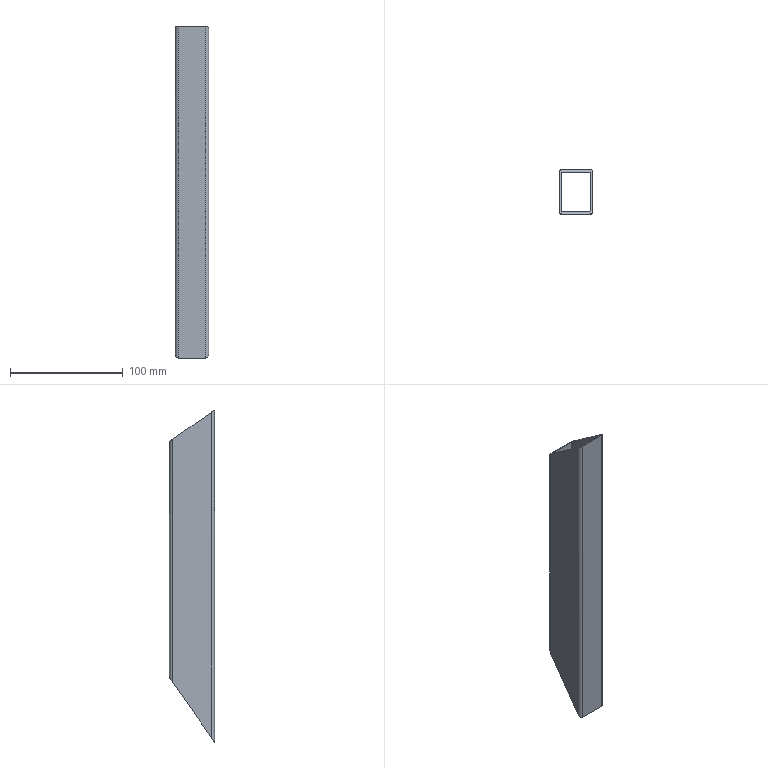Part | SolidWorks | features BaseBody 1 | 1 solid | 18 faces | box 30 x 40 x 295 mm | volume 80145 mm3 | plane 10 | cylinder 8 | commonest cylinder face diameters 1 x4 6 x4
STEP:
#1=CARTESIAN_POINT('',(-15.,17.,121.592));
#2=VERTEX_POINT('',#1);
#3=CARTESIAN_POINT('',(-15.,17.,-94.659));
#4=VERTEX_POINT('',#3);
#5=CARTESIAN_POINT('',(-15.,17.,147.5));
#6=DIRECTION('',(0.,0.,-1.));
#7=VECTOR('',#6,1000.);
#8=LINE('',#5,#7);
#9=EDGE_CURVE('',#2,#4,#8,.T.);
#10=ORIENTED_EDGE('',*,*,#9,.T.);
#11=CARTESIAN_POINT('',(-15.,-17.,-143.216));
#12=VERTEX_POINT('',#11);
#13=CARTESIAN_POINT('',(-15.,-20.,-147.5));
#14=DIRECTION('',(0.,0.5736,0.8192));
#15=VECTOR('',#14,1000.);
#16=LINE('',#13,#15);
#17=EDGE_CURVE('',#12,#4,#16,.T.);
#18=ORIENTED_EDGE('',*,*,#17,.F.);
#19=CARTESIAN_POINT('',(-15.,-17.,145.399));
#20=VERTEX_POINT('',#19);
#21=CARTESIAN_POINT('',(-15.,-17.,147.5));
#22=DIRECTION('',(0.,0.,-1.));
#23=VECTOR('',#22,1000.);
#24=LINE('',#21,#23);
#25=EDGE_CURVE('',#20,#12,#24,.T.);
#26=ORIENTED_EDGE('',*,*,#25,.F.);
#27=CARTESIAN_POINT('',(-15.,-20.,147.5));
#28=DIRECTION('',(0.,-0.8192,0.5736));
#29=VECTOR('',#28,1000.);
#30=LINE('',#27,#29);
#31=EDGE_CURVE('',#2,#20,#30,.T.);
#32=ORIENTED_EDGE('',*,*,#31,.F.);
#33=EDGE_LOOP('',(#10,#18,#26,#32));
#34=FACE_OUTER_BOUND('',#33,.T.);
#35=CARTESIAN_POINT('',(-15.,17.,147.5));
#36=DIRECTION('',(1.,0.,0.));
#37=DIRECTION('',(0.,1.,0.));
#38=AXIS2_PLACEMENT_3D('',#35,#36,#37);
#39=PLANE('',#38);
#40=ADVANCED_FACE('',(#34),#39,.F.);
#41=CARTESIAN_POINT('',(-12.,20.,119.492));
#42=VERTEX_POINT('',#41);
#43=CARTESIAN_POINT('',(-12.,20.,-90.374));
#44=VERTEX_POINT('',#43);
#45=CARTESIAN_POINT('',(-12.,20.,147.5));
#46=DIRECTION('',(0.,0.,-1.));
#47=VECTOR('',#46,1000.);
#48=LINE('',#45,#47);
#49=EDGE_CURVE('',#42,#44,#48,.T.);
#50=ORIENTED_EDGE('',*,*,#49,.T.);
#51=CARTESIAN_POINT('',(-12.,20.,-90.374));
#52=CARTESIAN_POINT('',(-13.757,20.,-90.374));
#53=CARTESIAN_POINT('',(-15.,18.757,-92.149));
#54=CARTESIAN_POINT('',(-15.,17.,-94.659));
#55=(BOUNDED_CURVE()B_SPLINE_CURVE(3,(#51,#52,#53,#54),.UNSPECIFIED.,.F.,.T.)B_SPLINE_CURVE_WITH_KNOTS((4,4),(3.142,4.712),.UNSPECIFIED.)CURVE()GEOMETRIC_REPRESENTATION_ITEM()RATIONAL_B_SPLINE_CURVE((1.,0.8047,0.8047,1.))REPRESENTATION_ITEM(''));
#56=EDGE_CURVE('',#44,#4,#55,.T.);
#57=ORIENTED_EDGE('',*,*,#56,.T.);
#58=ORIENTED_EDGE('',*,*,#9,.F.);
#59=CARTESIAN_POINT('',(-15.,17.,121.592));
#60=CARTESIAN_POINT('',(-15.,18.757,120.362));
#61=CARTESIAN_POINT('',(-13.757,20.,119.492));
#62=CARTESIAN_POINT('',(-12.,20.,119.492));
#63=(BOUNDED_CURVE()B_SPLINE_CURVE(3,(#59,#60,#61,#62),.UNSPECIFIED.,.F.,.F.)B_SPLINE_CURVE_WITH_KNOTS((4,4),(4.712,6.283),.UNSPECIFIED.)CURVE()GEOMETRIC_REPRESENTATION_ITEM()RATIONAL_B_SPLINE_CURVE((1.,0.8047,0.8047,1.))REPRESENTATION_ITEM(''));
#64=EDGE_CURVE('',#2,#42,#63,.T.);
#65=ORIENTED_EDGE('',*,*,#64,.T.);
#66=EDGE_LOOP('',(#50,#57,#58,#65));
#67=FACE_OUTER_BOUND('',#66,.T.);
#68=CARTESIAN_POINT('',(-12.,17.,147.5));
#69=DIRECTION('',(0.,0.,-1.));
#70=DIRECTION('',(-1.,0.,0.));
#71=AXIS2_PLACEMENT_3D('',#68,#69,#70);
#72=CYLINDRICAL_SURFACE('',#71,3.);
#73=ADVANCED_FACE('',(#67),#72,.T.);
#74=CARTESIAN_POINT('',(12.,20.,119.492));
#75=VERTEX_POINT('',#74);
#76=CARTESIAN_POINT('',(12.,20.,-90.374));
#77=VERTEX_POINT('',#76);
#78=CARTESIAN_POINT('',(12.,20.,147.5));
#79=DIRECTION('',(0.,0.,-1.));
#80=VECTOR('',#79,1000.);
#81=LINE('',#78,#80);
#82=EDGE_CURVE('',#75,#77,#81,.T.);
#83=ORIENTED_EDGE('',*,*,#82,.T.);
#84=CARTESIAN_POINT('',(15.,20.,-90.374));
#85=DIRECTION('',(-1.,0.,0.));
#86=VECTOR('',#85,1000.);
#87=LINE('',#84,#86);
#88=EDGE_CURVE('',#77,#44,#87,.T.);
#89=ORIENTED_EDGE('',*,*,#88,.T.);
#90=ORIENTED_EDGE('',*,*,#49,.F.);
#91=CARTESIAN_POINT('',(15.,20.,119.492));
#92=DIRECTION('',(-1.,0.,0.));
#93=VECTOR('',#92,1000.);
#94=LINE('',#91,#93);
#95=EDGE_CURVE('',#75,#42,#94,.T.);
#96=ORIENTED_EDGE('',*,*,#95,.F.);
#97=EDGE_LOOP('',(#83,#89,#90,#96));
#98=FACE_OUTER_BOUND('',#97,.T.);
#99=CARTESIAN_POINT('',(-12.,20.,147.5));
#100=DIRECTION('',(0.,-1.,0.));
#101=DIRECTION('',(0.,0.,-1.));
#102=AXIS2_PLACEMENT_3D('',#99,#100,#101);
#103=PLANE('',#102);
#104=ADVANCED_FACE('',(#98),#103,.F.);
#105=CARTESIAN_POINT('',(15.,17.,121.592));
#106=VERTEX_POINT('',#105);
#107=CARTESIAN_POINT('',(15.,17.,-94.659));
#108=VERTEX_POINT('',#107);
#109=CARTESIAN_POINT('',(15.,17.,147.5));
#110=DIRECTION('',(0.,0.,-1.));
#111=VECTOR('',#110,1000.);
#112=LINE('',#109,#111);
#113=EDGE_CURVE('',#106,#108,#112,.T.);
#114=ORIENTED_EDGE('',*,*,#113,.T.);
#115=CARTESIAN_POINT('',(15.,17.,-94.659));
#116=CARTESIAN_POINT('',(15.,18.757,-92.149));
#117=CARTESIAN_POINT('',(13.757,20.,-90.374));
#118=CARTESIAN_POINT('',(12.,20.,-90.374));
#119=(BOUNDED_CURVE()B_SPLINE_CURVE(3,(#115,#116,#117,#118),.UNSPECIFIED.,.F.,.F.)B_SPLINE_CURVE_WITH_KNOTS((4,4),(1.571,3.142),.UNSPECIFIED.)CURVE()GEOMETRIC_REPRESENTATION_ITEM()RATIONAL_B_SPLINE_CURVE((1.,0.8047,0.8047,1.))REPRESENTATION_ITEM(''));
#120=EDGE_CURVE('',#108,#77,#119,.T.);
#121=ORIENTED_EDGE('',*,*,#120,.T.);
#122=ORIENTED_EDGE('',*,*,#82,.F.);
#123=CARTESIAN_POINT('',(12.,20.,119.492));
#124=CARTESIAN_POINT('',(13.757,20.,119.492));
#125=CARTESIAN_POINT('',(15.,18.757,120.362));
#126=CARTESIAN_POINT('',(15.,17.,121.592));
#127=(BOUNDED_CURVE()B_SPLINE_CURVE(3,(#123,#124,#125,#126),.UNSPECIFIED.,.F.,.F.)B_SPLINE_CURVE_WITH_KNOTS((4,4),(0.,1.571),.UNSPECIFIED.)CURVE()GEOMETRIC_REPRESENTATION_ITEM()RATIONAL_B_SPLINE_CURVE((1.,0.8047,0.8047,1.))REPRESENTATION_ITEM(''));
#128=EDGE_CURVE('',#75,#106,#127,.T.);
#129=ORIENTED_EDGE('',*,*,#128,.T.);
#130=EDGE_LOOP('',(#114,#121,#122,#129));
#131=FACE_OUTER_BOUND('',#130,.T.);
#132=CARTESIAN_POINT('',(12.,17.,147.5));
#133=DIRECTION('',(0.,0.,-1.));
#134=DIRECTION('',(-1.,0.,0.));
#135=AXIS2_PLACEMENT_3D('',#132,#133,#134);
#136=CYLINDRICAL_SURFACE('',#135,3.);
#137=ADVANCED_FACE('',(#131),#136,.T.);
#138=CARTESIAN_POINT('',(15.,-17.,145.399));
#139=VERTEX_POINT('',#138);
#140=CARTESIAN_POINT('',(15.,-17.,-143.216));
#141=VERTEX_POINT('',#140);
#142=CARTESIAN_POINT('',(15.,-17.,147.5));
#143=DIRECTION('',(0.,0.,-1.));
#144=VECTOR('',#143,1000.);
#145=LINE('',#142,#144);
#146=EDGE_CURVE('',#139,#141,#145,.T.);
#147=ORIENTED_EDGE('',*,*,#146,.T.);
#148=CARTESIAN_POINT('',(15.,-20.,-147.5));
#149=DIRECTION('',(0.,0.5736,0.8192));
#150=VECTOR('',#149,1000.);
#151=LINE('',#148,#150);
#152=EDGE_CURVE('',#141,#108,#151,.T.);
#153=ORIENTED_EDGE('',*,*,#152,.T.);
#154=ORIENTED_EDGE('',*,*,#113,.F.);
#155=CARTESIAN_POINT('',(15.,-20.,147.5));
#156=DIRECTION('',(0.,-0.8192,0.5736));
#157=VECTOR('',#156,1000.);
#158=LINE('',#155,#157);
#159=EDGE_CURVE('',#106,#139,#158,.T.);
#160=ORIENTED_EDGE('',*,*,#159,.T.);
#161=EDGE_LOOP('',(#147,#153,#154,#160));
#162=FACE_OUTER_BOUND('',#161,.T.);
#163=CARTESIAN_POINT('',(15.,17.,147.5));
#164=DIRECTION('',(-1.,0.,0.));
#165=DIRECTION('',(0.,1.,0.));
#166=AXIS2_PLACEMENT_3D('',#163,#164,#165);
#167=PLANE('',#166);
#168=ADVANCED_FACE('',(#162),#167,.F.);
#169=CARTESIAN_POINT('',(12.,-20.,147.5));
#170=VERTEX_POINT('',#169);
#171=CARTESIAN_POINT('',(12.,-20.,-147.5));
#172=VERTEX_POINT('',#171);
#173=CARTESIAN_POINT('',(12.,-20.,147.5));
#174=DIRECTION('',(0.,0.,-1.));
#175=VECTOR('',#174,1000.);
#176=LINE('',#173,#175);
#177=EDGE_CURVE('',#170,#172,#176,.T.);
#178=ORIENTED_EDGE('',*,*,#177,.T.);
#179=CARTESIAN_POINT('',(12.,-20.,-147.5));
#180=CARTESIAN_POINT('',(13.757,-20.,-147.5));
#181=CARTESIAN_POINT('',(15.,-18.757,-145.725));
#182=CARTESIAN_POINT('',(15.,-17.,-143.216));
#183=(BOUNDED_CURVE()B_SPLINE_CURVE(3,(#179,#180,#181,#182),.UNSPECIFIED.,.F.,.F.)B_SPLINE_CURVE_WITH_KNOTS((4,4),(0.,1.571),.UNSPECIFIED.)CURVE()GEOMETRIC_REPRESENTATION_ITEM()RATIONAL_B_SPLINE_CURVE((1.,0.8047,0.8047,1.))REPRESENTATION_ITEM(''));
#184=EDGE_CURVE('',#172,#141,#183,.T.);
#185=ORIENTED_EDGE('',*,*,#184,.T.);
#186=ORIENTED_EDGE('',*,*,#146,.F.);
#187=CARTESIAN_POINT('',(15.,-17.,145.399));
#188=CARTESIAN_POINT('',(15.,-18.757,146.63));
#189=CARTESIAN_POINT('',(13.757,-20.,147.5));
#190=CARTESIAN_POINT('',(12.,-20.,147.5));
#191=(BOUNDED_CURVE()B_SPLINE_CURVE(3,(#187,#188,#189,#190),.UNSPECIFIED.,.F.,.F.)B_SPLINE_CURVE_WITH_KNOTS((4,4),(1.571,3.142),.UNSPECIFIED.)CURVE()GEOMETRIC_REPRESENTATION_ITEM()RATIONAL_B_SPLINE_CURVE((1.,0.8047,0.8047,1.))REPRESENTATION_ITEM(''));
#192=EDGE_CURVE('',#139,#170,#191,.T.);
#193=ORIENTED_EDGE('',*,*,#192,.T.);
#194=EDGE_LOOP('',(#178,#185,#186,#193));
#195=FACE_OUTER_BOUND('',#194,.T.);
#196=CARTESIAN_POINT('',(12.,-17.,147.5));
#197=DIRECTION('',(0.,0.,-1.));
#198=DIRECTION('',(-1.,0.,0.));
#199=AXIS2_PLACEMENT_3D('',#196,#197,#198);
#200=CYLINDRICAL_SURFACE('',#199,3.);
#201=ADVANCED_FACE('',(#195),#200,.T.);
#202=CARTESIAN_POINT('',(-12.,-20.,-147.5));
#203=VERTEX_POINT('',#202);
#204=CARTESIAN_POINT('',(-12.,-20.,-147.5));
#205=DIRECTION('',(1.,0.,0.));
#206=VECTOR('',#205,1000.);
#207=LINE('',#204,#206);
#208=EDGE_CURVE('',#203,#172,#207,.T.);
#209=ORIENTED_EDGE('',*,*,#208,.T.);
#210=ORIENTED_EDGE('',*,*,#177,.F.);
#211=CARTESIAN_POINT('',(-12.,-20.,147.5));
#212=VERTEX_POINT('',#211);
#213=CARTESIAN_POINT('',(-12.,-20.,147.5));
#214=DIRECTION('',(1.,0.,0.));
#215=VECTOR('',#214,1000.);
#216=LINE('',#213,#215);
#217=EDGE_CURVE('',#212,#170,#216,.T.);
#218=ORIENTED_EDGE('',*,*,#217,.F.);
#219=CARTESIAN_POINT('',(-12.,-20.,147.5));
#220=DIRECTION('',(0.,0.,-1.));
#221=VECTOR('',#220,1000.);
#222=LINE('',#219,#221);
#223=EDGE_CURVE('',#212,#203,#222,.T.);
#224=ORIENTED_EDGE('',*,*,#223,.T.);
#225=EDGE_LOOP('',(#209,#210,#218,#224));
#226=FACE_OUTER_BOUND('',#225,.T.);
#227=CARTESIAN_POINT('',(-12.,-20.,147.5));
#228=DIRECTION('',(0.,1.,0.));
#229=DIRECTION('',(1.,0.,0.));
#230=AXIS2_PLACEMENT_3D('',#227,#228,#229);
#231=PLANE('',#230);
#232=ADVANCED_FACE('',(#226),#231,.F.);
#233=ORIENTED_EDGE('',*,*,#25,.T.);
#234=CARTESIAN_POINT('',(-15.,-17.,-143.216));
#235=CARTESIAN_POINT('',(-15.,-18.757,-145.725));
#236=CARTESIAN_POINT('',(-13.757,-20.,-147.5));
#237=CARTESIAN_POINT('',(-12.,-20.,-147.5));
#238=(BOUNDED_CURVE()B_SPLINE_CURVE(3,(#234,#235,#236,#237),.UNSPECIFIED.,.F.,.F.)B_SPLINE_CURVE_WITH_KNOTS((4,4),(4.712,6.283),.UNSPECIFIED.)CURVE()GEOMETRIC_REPRESENTATION_ITEM()RATIONAL_B_SPLINE_CURVE((1.,0.8047,0.8047,1.))REPRESENTATION_ITEM(''));
#239=EDGE_CURVE('',#12,#203,#238,.T.);
#240=ORIENTED_EDGE('',*,*,#239,.T.);
#241=ORIENTED_EDGE('',*,*,#223,.F.);
#242=CARTESIAN_POINT('',(-12.,-20.,147.5));
#243=CARTESIAN_POINT('',(-13.757,-20.,147.5));
#244=CARTESIAN_POINT('',(-15.,-18.757,146.63));
#245=CARTESIAN_POINT('',(-15.,-17.,145.399));
#246=(BOUNDED_CURVE()B_SPLINE_CURVE(3,(#242,#243,#244,#245),.UNSPECIFIED.,.F.,.F.)B_SPLINE_CURVE_WITH_KNOTS((4,4),(3.142,4.712),.UNSPECIFIED.)CURVE()GEOMETRIC_REPRESENTATION_ITEM()RATIONAL_B_SPLINE_CURVE((1.,0.8047,0.8047,1.))REPRESENTATION_ITEM(''));
#247=EDGE_CURVE('',#212,#20,#246,.T.);
#248=ORIENTED_EDGE('',*,*,#247,.T.);
#249=EDGE_LOOP('',(#233,#240,#241,#248));
#250=FACE_OUTER_BOUND('',#249,.T.);
#251=CARTESIAN_POINT('',(-12.,-17.,147.5));
#252=DIRECTION('',(0.,0.,-1.));
#253=DIRECTION('',(-1.,0.,0.));
#254=AXIS2_PLACEMENT_3D('',#251,#252,#253);
#255=CYLINDRICAL_SURFACE('',#254,3.);
#256=ADVANCED_FACE('',(#250),#255,.T.);
#257=CARTESIAN_POINT('',(-12.,17.5,-93.944));
#258=VERTEX_POINT('',#257);
#259=CARTESIAN_POINT('',(-12.5,17.,-94.659));
#260=VERTEX_POINT('',#259);
#261=CARTESIAN_POINT('',(-12.,17.5,-93.944));
#262=CARTESIAN_POINT('',(-12.293,17.5,-93.944));
#263=CARTESIAN_POINT('',(-12.5,17.293,-94.24));
#264=CARTESIAN_POINT('',(-12.5,17.,-94.659));
#265=(BOUNDED_CURVE()B_SPLINE_CURVE(3,(#261,#262,#263,#264),.UNSPECIFIED.,.F.,.F.)B_SPLINE_CURVE_WITH_KNOTS((4,4),(3.142,4.712),.UNSPECIFIED.)CURVE()GEOMETRIC_REPRESENTATION_ITEM()RATIONAL_B_SPLINE_CURVE((1.,0.8047,0.8047,1.))REPRESENTATION_ITEM(''));
#266=EDGE_CURVE('',#258,#260,#265,.T.);
#267=ORIENTED_EDGE('',*,*,#266,.T.);
#268=CARTESIAN_POINT('',(-12.5,-17.,-143.216));
#269=VERTEX_POINT('',#268);
#270=CARTESIAN_POINT('',(-12.5,130.777,67.832));
#271=DIRECTION('',(0.,-0.5736,-0.8192));
#272=VECTOR('',#271,1000.);
#273=LINE('',#270,#272);
#274=EDGE_CURVE('',#260,#269,#273,.T.);
#275=ORIENTED_EDGE('',*,*,#274,.T.);
#276=CARTESIAN_POINT('',(-12.,-17.5,-143.93));
#277=VERTEX_POINT('',#276);
#278=CARTESIAN_POINT('',(-12.5,-17.,-143.216));
#279=CARTESIAN_POINT('',(-12.5,-17.293,-143.634));
#280=CARTESIAN_POINT('',(-12.293,-17.5,-143.93));
#281=CARTESIAN_POINT('',(-12.,-17.5,-143.93));
#282=(BOUNDED_CURVE()B_SPLINE_CURVE(3,(#278,#279,#280,#281),.UNSPECIFIED.,.F.,.F.)B_SPLINE_CURVE_WITH_KNOTS((4,4),(4.712,6.283),.UNSPECIFIED.)CURVE()GEOMETRIC_REPRESENTATION_ITEM()RATIONAL_B_SPLINE_CURVE((1.,0.8047,0.8047,1.))REPRESENTATION_ITEM(''));
#283=EDGE_CURVE('',#269,#277,#282,.T.);
#284=ORIENTED_EDGE('',*,*,#283,.T.);
#285=CARTESIAN_POINT('',(12.,-17.5,-143.93));
#286=VERTEX_POINT('',#285);
#287=CARTESIAN_POINT('',(-12.,-17.5,-143.93));
#288=DIRECTION('',(1.,0.,0.));
#289=VECTOR('',#288,1000.);
#290=LINE('',#287,#289);
#291=EDGE_CURVE('',#277,#286,#290,.T.);
#292=ORIENTED_EDGE('',*,*,#291,.T.);
#293=CARTESIAN_POINT('',(12.5,-17.,-143.216));
#294=VERTEX_POINT('',#293);
#295=CARTESIAN_POINT('',(12.,-17.5,-143.93));
#296=CARTESIAN_POINT('',(12.293,-17.5,-143.93));
#297=CARTESIAN_POINT('',(12.5,-17.293,-143.634));
#298=CARTESIAN_POINT('',(12.5,-17.,-143.216));
#299=(BOUNDED_CURVE()B_SPLINE_CURVE(3,(#295,#296,#297,#298),.UNSPECIFIED.,.F.,.F.)B_SPLINE_CURVE_WITH_KNOTS((4,4),(0.,1.571),.UNSPECIFIED.)CURVE()GEOMETRIC_REPRESENTATION_ITEM()RATIONAL_B_SPLINE_CURVE((1.,0.8047,0.8047,1.))REPRESENTATION_ITEM(''));
#300=EDGE_CURVE('',#286,#294,#299,.T.);
#301=ORIENTED_EDGE('',*,*,#300,.T.);
#302=CARTESIAN_POINT('',(12.5,17.,-94.659));
#303=VERTEX_POINT('',#302);
#304=CARTESIAN_POINT('',(12.5,130.777,67.832));
#305=DIRECTION('',(0.,0.5736,0.8192));
#306=VECTOR('',#305,1000.);
#307=LINE('',#304,#306);
#308=EDGE_CURVE('',#294,#303,#307,.T.);
#309=ORIENTED_EDGE('',*,*,#308,.T.);
#310=CARTESIAN_POINT('',(12.,17.5,-93.944));
#311=VERTEX_POINT('',#310);
#312=CARTESIAN_POINT('',(12.5,17.,-94.659));
#313=CARTESIAN_POINT('',(12.5,17.293,-94.24));
#314=CARTESIAN_POINT('',(12.293,17.5,-93.944));
#315=CARTESIAN_POINT('',(12.,17.5,-93.944));
#316=(BOUNDED_CURVE()B_SPLINE_CURVE(3,(#312,#313,#314,#315),.UNSPECIFIED.,.F.,.T.)B_SPLINE_CURVE_WITH_KNOTS((4,4),(1.571,3.142),.UNSPECIFIED.)CURVE()GEOMETRIC_REPRESENTATION_ITEM()RATIONAL_B_SPLINE_CURVE((1.,0.8047,0.8047,1.))REPRESENTATION_ITEM(''));
#317=EDGE_CURVE('',#303,#311,#316,.T.);
#318=ORIENTED_EDGE('',*,*,#317,.T.);
#319=CARTESIAN_POINT('',(-12.,17.5,-93.944));
#320=DIRECTION('',(-1.,0.,0.));
#321=VECTOR('',#320,1000.);
#322=LINE('',#319,#321);
#323=EDGE_CURVE('',#311,#258,#322,.T.);
#324=ORIENTED_EDGE('',*,*,#323,.T.);
#325=EDGE_LOOP('',(#267,#275,#284,#292,#301,#309,#318,#324));
#326=FACE_BOUND('',#325,.T.);
#327=ORIENTED_EDGE('',*,*,#17,.T.);
#328=ORIENTED_EDGE('',*,*,#56,.F.);
#329=ORIENTED_EDGE('',*,*,#88,.F.);
#330=ORIENTED_EDGE('',*,*,#120,.F.);
#331=ORIENTED_EDGE('',*,*,#152,.F.);
#332=ORIENTED_EDGE('',*,*,#184,.F.);
#333=ORIENTED_EDGE('',*,*,#208,.F.);
#334=ORIENTED_EDGE('',*,*,#239,.F.);
#335=EDGE_LOOP('',(#327,#328,#329,#330,#331,#332,#333,#334));
#336=FACE_OUTER_BOUND('',#335,.T.);
#337=CARTESIAN_POINT('',(15.,-20.,-147.5));
#338=DIRECTION('',(0.,-0.8192,0.5736));
#339=DIRECTION('',(-1.,0.,0.));
#340=AXIS2_PLACEMENT_3D('',#337,#338,#339);
#341=PLANE('',#340);
#342=ADVANCED_FACE('',(#326,#336),#341,.F.);
#343=CARTESIAN_POINT('',(-12.5,17.,121.592));
#344=VERTEX_POINT('',#343);
#345=CARTESIAN_POINT('',(-12.,17.5,121.242));
#346=VERTEX_POINT('',#345);
#347=CARTESIAN_POINT('',(-12.5,17.,121.592));
#348=CARTESIAN_POINT('',(-12.5,17.293,121.387));
#349=CARTESIAN_POINT('',(-12.293,17.5,121.242));
#350=CARTESIAN_POINT('',(-12.,17.5,121.242));
#351=(BOUNDED_CURVE()B_SPLINE_CURVE(3,(#347,#348,#349,#350),.UNSPECIFIED.,.F.,.F.)B_SPLINE_CURVE_WITH_KNOTS((4,4),(4.712,6.283),.UNSPECIFIED.)CURVE()GEOMETRIC_REPRESENTATION_ITEM()RATIONAL_B_SPLINE_CURVE((1.,0.8047,0.8047,1.))REPRESENTATION_ITEM(''));
#352=EDGE_CURVE('',#344,#346,#351,.T.);
#353=ORIENTED_EDGE('',*,*,#352,.T.);
#354=CARTESIAN_POINT('',(12.,17.5,121.242));
#355=VERTEX_POINT('',#354);
#356=CARTESIAN_POINT('',(-12.,17.5,121.242));
#357=DIRECTION('',(1.,0.,0.));
#358=VECTOR('',#357,1000.);
#359=LINE('',#356,#358);
#360=EDGE_CURVE('',#346,#355,#359,.T.);
#361=ORIENTED_EDGE('',*,*,#360,.T.);
#362=CARTESIAN_POINT('',(12.5,17.,121.592));
#363=VERTEX_POINT('',#362);
#364=CARTESIAN_POINT('',(12.,17.5,121.242));
#365=CARTESIAN_POINT('',(12.293,17.5,121.242));
#366=CARTESIAN_POINT('',(12.5,17.293,121.387));
#367=CARTESIAN_POINT('',(12.5,17.,121.592));
#368=(BOUNDED_CURVE()B_SPLINE_CURVE(3,(#364,#365,#366,#367),.UNSPECIFIED.,.F.,.F.)B_SPLINE_CURVE_WITH_KNOTS((4,4),(0.,1.571),.UNSPECIFIED.)CURVE()GEOMETRIC_REPRESENTATION_ITEM()RATIONAL_B_SPLINE_CURVE((1.,0.8047,0.8047,1.))REPRESENTATION_ITEM(''));
#369=EDGE_CURVE('',#355,#363,#368,.T.);
#370=ORIENTED_EDGE('',*,*,#369,.T.);
#371=CARTESIAN_POINT('',(12.5,-17.,145.399));
#372=VERTEX_POINT('',#371);
#373=CARTESIAN_POINT('',(12.5,4.827,130.116));
#374=DIRECTION('',(0.,-0.8192,0.5736));
#375=VECTOR('',#374,1000.);
#376=LINE('',#373,#375);
#377=EDGE_CURVE('',#363,#372,#376,.T.);
#378=ORIENTED_EDGE('',*,*,#377,.T.);
#379=CARTESIAN_POINT('',(12.,-17.5,145.749));
#380=VERTEX_POINT('',#379);
#381=CARTESIAN_POINT('',(12.5,-17.,145.399));
#382=CARTESIAN_POINT('',(12.5,-17.293,145.604));
#383=CARTESIAN_POINT('',(12.293,-17.5,145.749));
#384=CARTESIAN_POINT('',(12.,-17.5,145.749));
#385=(BOUNDED_CURVE()B_SPLINE_CURVE(3,(#381,#382,#383,#384),.UNSPECIFIED.,.F.,.F.)B_SPLINE_CURVE_WITH_KNOTS((4,4),(1.571,3.142),.UNSPECIFIED.)CURVE()GEOMETRIC_REPRESENTATION_ITEM()RATIONAL_B_SPLINE_CURVE((1.,0.8047,0.8047,1.))REPRESENTATION_ITEM(''));
#386=EDGE_CURVE('',#372,#380,#385,.T.);
#387=ORIENTED_EDGE('',*,*,#386,.T.);
#388=CARTESIAN_POINT('',(-12.,-17.5,145.749));
#389=VERTEX_POINT('',#388);
#390=CARTESIAN_POINT('',(-12.,-17.5,145.749));
#391=DIRECTION('',(-1.,0.,0.));
#392=VECTOR('',#391,1000.);
#393=LINE('',#390,#392);
#394=EDGE_CURVE('',#380,#389,#393,.T.);
#395=ORIENTED_EDGE('',*,*,#394,.T.);
#396=CARTESIAN_POINT('',(-12.5,-17.,145.399));
#397=VERTEX_POINT('',#396);
#398=CARTESIAN_POINT('',(-12.,-17.5,145.749));
#399=CARTESIAN_POINT('',(-12.293,-17.5,145.749));
#400=CARTESIAN_POINT('',(-12.5,-17.293,145.604));
#401=CARTESIAN_POINT('',(-12.5,-17.,145.399));
#402=(BOUNDED_CURVE()B_SPLINE_CURVE(3,(#398,#399,#400,#401),.UNSPECIFIED.,.F.,.F.)B_SPLINE_CURVE_WITH_KNOTS((4,4),(3.142,4.712),.UNSPECIFIED.)CURVE()GEOMETRIC_REPRESENTATION_ITEM()RATIONAL_B_SPLINE_CURVE((1.,0.8047,0.8047,1.))REPRESENTATION_ITEM(''));
#403=EDGE_CURVE('',#389,#397,#402,.T.);
#404=ORIENTED_EDGE('',*,*,#403,.T.);
#405=CARTESIAN_POINT('',(-12.5,4.827,130.116));
#406=DIRECTION('',(0.,0.8192,-0.5736));
#407=VECTOR('',#406,1000.);
#408=LINE('',#405,#407);
#409=EDGE_CURVE('',#397,#344,#408,.T.);
#410=ORIENTED_EDGE('',*,*,#409,.T.);
#411=EDGE_LOOP('',(#353,#361,#370,#378,#387,#395,#404,#410));
#412=FACE_BOUND('',#411,.T.);
#413=ORIENTED_EDGE('',*,*,#217,.T.);
#414=ORIENTED_EDGE('',*,*,#192,.F.);
#415=ORIENTED_EDGE('',*,*,#159,.F.);
#416=ORIENTED_EDGE('',*,*,#128,.F.);
#417=ORIENTED_EDGE('',*,*,#95,.T.);
#418=ORIENTED_EDGE('',*,*,#64,.F.);
#419=ORIENTED_EDGE('',*,*,#31,.T.);
#420=ORIENTED_EDGE('',*,*,#247,.F.);
#421=EDGE_LOOP('',(#413,#414,#415,#416,#417,#418,#419,#420));
#422=FACE_OUTER_BOUND('',#421,.T.);
#423=CARTESIAN_POINT('',(15.,-20.,147.5));
#424=DIRECTION('',(0.,-0.5736,-0.8192));
#425=DIRECTION('',(0.,-0.8192,0.5736));
#426=AXIS2_PLACEMENT_3D('',#423,#424,#425);
#427=PLANE('',#426);
#428=ADVANCED_FACE('',(#412,#422),#427,.F.);
#429=ORIENTED_EDGE('',*,*,#266,.F.);
#430=CARTESIAN_POINT('',(-12.,17.5,147.5));
#431=DIRECTION('',(0.,0.,-1.));
#432=VECTOR('',#431,1000.);
#433=LINE('',#430,#432);
#434=EDGE_CURVE('',#346,#258,#433,.T.);
#435=ORIENTED_EDGE('',*,*,#434,.F.);
#436=ORIENTED_EDGE('',*,*,#352,.F.);
#437=CARTESIAN_POINT('',(-12.5,17.,147.5));
#438=DIRECTION('',(0.,0.,-1.));
#439=VECTOR('',#438,1000.);
#440=LINE('',#437,#439);
#441=EDGE_CURVE('',#344,#260,#440,.T.);
#442=ORIENTED_EDGE('',*,*,#441,.T.);
#443=EDGE_LOOP('',(#429,#435,#436,#442));
#444=FACE_OUTER_BOUND('',#443,.T.);
#445=CARTESIAN_POINT('',(-12.,17.,147.5));
#446=DIRECTION('',(0.,0.,-1.));
#447=DIRECTION('',(-1.,0.,0.));
#448=AXIS2_PLACEMENT_3D('',#445,#446,#447);
#449=CYLINDRICAL_SURFACE('',#448,0.5);
#450=ADVANCED_FACE('',(#444),#449,.F.);
#451=ORIENTED_EDGE('',*,*,#274,.F.);
#452=ORIENTED_EDGE('',*,*,#441,.F.);
#453=ORIENTED_EDGE('',*,*,#409,.F.);
#454=CARTESIAN_POINT('',(-12.5,-17.,147.5));
#455=DIRECTION('',(0.,0.,-1.));
#456=VECTOR('',#455,1000.);
#457=LINE('',#454,#456);
#458=EDGE_CURVE('',#397,#269,#457,.T.);
#459=ORIENTED_EDGE('',*,*,#458,.T.);
#460=EDGE_LOOP('',(#451,#452,#453,#459));
#461=FACE_OUTER_BOUND('',#460,.T.);
#462=CARTESIAN_POINT('',(-12.5,17.,147.5));
#463=DIRECTION('',(1.,0.,0.));
#464=DIRECTION('',(0.,1.,0.));
#465=AXIS2_PLACEMENT_3D('',#462,#463,#464);
#466=PLANE('',#465);
#467=ADVANCED_FACE('',(#461),#466,.T.);
#468=ORIENTED_EDGE('',*,*,#283,.F.);
#469=ORIENTED_EDGE('',*,*,#458,.F.);
#470=ORIENTED_EDGE('',*,*,#403,.F.);
#471=CARTESIAN_POINT('',(-12.,-17.5,147.5));
#472=DIRECTION('',(0.,0.,-1.));
#473=VECTOR('',#472,1000.);
#474=LINE('',#471,#473);
#475=EDGE_CURVE('',#389,#277,#474,.T.);
#476=ORIENTED_EDGE('',*,*,#475,.T.);
#477=EDGE_LOOP('',(#468,#469,#470,#476));
#478=FACE_OUTER_BOUND('',#477,.T.);
#479=CARTESIAN_POINT('',(-12.,-17.,147.5));
#480=DIRECTION('',(0.,0.,-1.));
#481=DIRECTION('',(-1.,0.,0.));
#482=AXIS2_PLACEMENT_3D('',#479,#480,#481);
#483=CYLINDRICAL_SURFACE('',#482,0.5);
#484=ADVANCED_FACE('',(#478),#483,.F.);
#485=ORIENTED_EDGE('',*,*,#291,.F.);
#486=ORIENTED_EDGE('',*,*,#475,.F.);
#487=ORIENTED_EDGE('',*,*,#394,.F.);
#488=CARTESIAN_POINT('',(12.,-17.5,147.5));
#489=DIRECTION('',(0.,0.,-1.));
#490=VECTOR('',#489,1000.);
#491=LINE('',#488,#490);
#492=EDGE_CURVE('',#380,#286,#491,.T.);
#493=ORIENTED_EDGE('',*,*,#492,.T.);
#494=EDGE_LOOP('',(#485,#486,#487,#493));
#495=FACE_OUTER_BOUND('',#494,.T.);
#496=CARTESIAN_POINT('',(-12.,-17.5,147.5));
#497=DIRECTION('',(0.,1.,0.));
#498=DIRECTION('',(1.,0.,0.));
#499=AXIS2_PLACEMENT_3D('',#496,#497,#498);
#500=PLANE('',#499);
#501=ADVANCED_FACE('',(#495),#500,.T.);
#502=ORIENTED_EDGE('',*,*,#300,.F.);
#503=ORIENTED_EDGE('',*,*,#492,.F.);
#504=ORIENTED_EDGE('',*,*,#386,.F.);
#505=CARTESIAN_POINT('',(12.5,-17.,147.5));
#506=DIRECTION('',(0.,0.,-1.));
#507=VECTOR('',#506,1000.);
#508=LINE('',#505,#507);
#509=EDGE_CURVE('',#372,#294,#508,.T.);
#510=ORIENTED_EDGE('',*,*,#509,.T.);
#511=EDGE_LOOP('',(#502,#503,#504,#510));
#512=FACE_OUTER_BOUND('',#511,.T.);
#513=CARTESIAN_POINT('',(12.,-17.,147.5));
#514=DIRECTION('',(0.,0.,-1.));
#515=DIRECTION('',(-1.,0.,0.));
#516=AXIS2_PLACEMENT_3D('',#513,#514,#515);
#517=CYLINDRICAL_SURFACE('',#516,0.5);
#518=ADVANCED_FACE('',(#512),#517,.F.);
#519=ORIENTED_EDGE('',*,*,#308,.F.);
#520=ORIENTED_EDGE('',*,*,#509,.F.);
#521=ORIENTED_EDGE('',*,*,#377,.F.);
#522=CARTESIAN_POINT('',(12.5,17.,147.5));
#523=DIRECTION('',(0.,0.,-1.));
#524=VECTOR('',#523,1000.);
#525=LINE('',#522,#524);
#526=EDGE_CURVE('',#363,#303,#525,.T.);
#527=ORIENTED_EDGE('',*,*,#526,.T.);
#528=EDGE_LOOP('',(#519,#520,#521,#527));
#529=FACE_OUTER_BOUND('',#528,.T.);
#530=CARTESIAN_POINT('',(12.5,17.,147.5));
#531=DIRECTION('',(-1.,0.,0.));
#532=DIRECTION('',(0.,1.,0.));
#533=AXIS2_PLACEMENT_3D('',#530,#531,#532);
#534=PLANE('',#533);
#535=ADVANCED_FACE('',(#529),#534,.T.);
#536=ORIENTED_EDGE('',*,*,#317,.F.);
#537=ORIENTED_EDGE('',*,*,#526,.F.);
#538=ORIENTED_EDGE('',*,*,#369,.F.);
#539=CARTESIAN_POINT('',(12.,17.5,147.5));
#540=DIRECTION('',(0.,0.,-1.));
#541=VECTOR('',#540,1000.);
#542=LINE('',#539,#541);
#543=EDGE_CURVE('',#355,#311,#542,.T.);
#544=ORIENTED_EDGE('',*,*,#543,.T.);
#545=EDGE_LOOP('',(#536,#537,#538,#544));
#546=FACE_OUTER_BOUND('',#545,.T.);
#547=CARTESIAN_POINT('',(12.,17.,147.5));
#548=DIRECTION('',(0.,0.,-1.));
#549=DIRECTION('',(-1.,0.,0.));
#550=AXIS2_PLACEMENT_3D('',#547,#548,#549);
#551=CYLINDRICAL_SURFACE('',#550,0.5);
#552=ADVANCED_FACE('',(#546),#551,.F.);
#553=ORIENTED_EDGE('',*,*,#323,.F.);
#554=ORIENTED_EDGE('',*,*,#543,.F.);
#555=ORIENTED_EDGE('',*,*,#360,.F.);
#556=ORIENTED_EDGE('',*,*,#434,.T.);
#557=EDGE_LOOP('',(#553,#554,#555,#556));
#558=FACE_OUTER_BOUND('',#557,.T.);
#559=CARTESIAN_POINT('',(-12.,17.5,147.5));
#560=DIRECTION('',(0.,-1.,0.));
#561=DIRECTION('',(0.,0.,-1.));
#562=AXIS2_PLACEMENT_3D('',#559,#560,#561);
#563=PLANE('',#562);
#564=ADVANCED_FACE('',(#558),#563,.T.);
#565=CLOSED_SHELL('',(#40,#73,#104,#137,#168,#201,#232,#256,#342,#428,#450,#467,#484,#501,#518,#535,#552,#564));
#566=MANIFOLD_SOLID_BREP('',#565);
#567=CARTESIAN_POINT('',(0.,0.,0.));
#568=DIRECTION('',(0.,0.,1.));
#569=DIRECTION('',(1.,0.,0.));
#570=AXIS2_PLACEMENT_3D('',#567,#568,#569);
#571=(LENGTH_UNIT()NAMED_UNIT(*)SI_UNIT(.MILLI.,.METRE.));
#572=UNCERTAINTY_MEASURE_WITH_UNIT(LENGTH_MEASURE(0.00001),#571,'','');
#573=(NAMED_UNIT(*)PLANE_ANGLE_UNIT()SI_UNIT($,.RADIAN.));
#574=(NAMED_UNIT(*)SI_UNIT($,.STERADIAN.)SOLID_ANGLE_UNIT());
#575=(GEOMETRIC_REPRESENTATION_CONTEXT(3)GLOBAL_UNCERTAINTY_ASSIGNED_CONTEXT((#572))GLOBAL_UNIT_ASSIGNED_CONTEXT((#571,#573,#574))REPRESENTATION_CONTEXT('',''));
#576=ADVANCED_BREP_SHAPE_REPRESENTATION('',(#566,#570),#575);